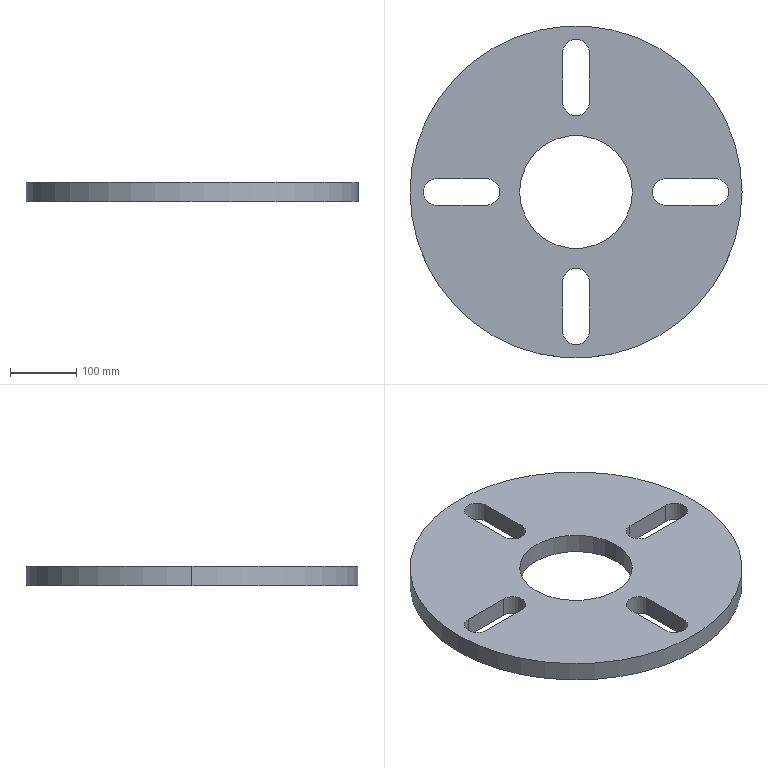Part | SolidWorks | features BaseBody 1 | 1 solid | 24 faces | box 500 x 500 x 30 mm | volume 4699230 mm3 | cylinder 14 | plane 10 | commonest cylinder face diameters 40 x10 170 x2 500 x2
STEP:
#1=CARTESIAN_POINT('',(2992.168,2025.631,30.));
#2=VERTEX_POINT('',#1);
#3=CARTESIAN_POINT('',(3162.168,2025.631,30.));
#4=VERTEX_POINT('',#3);
#5=CARTESIAN_POINT('',(3077.168,2025.631,30.));
#6=DIRECTION('',(0.,0.,1.));
#7=DIRECTION('',(1.,0.,0.));
#8=AXIS2_PLACEMENT_3D('',#5,#6,#7);
#9=CIRCLE('',#8,85.);
#10=EDGE_CURVE('',#2,#4,#9,.T.);
#11=ORIENTED_EDGE('',*,*,#10,.T.);
#12=CARTESIAN_POINT('',(3162.168,2025.631,0.));
#13=VERTEX_POINT('',#12);
#14=CARTESIAN_POINT('',(3162.168,2025.631,30.));
#15=DIRECTION('',(0.,0.,-1.));
#16=VECTOR('',#15,1000.);
#17=LINE('',#14,#16);
#18=EDGE_CURVE('',#4,#13,#17,.T.);
#19=ORIENTED_EDGE('',*,*,#18,.T.);
#20=CARTESIAN_POINT('',(2992.168,2025.631,0.));
#21=VERTEX_POINT('',#20);
#22=CARTESIAN_POINT('',(3077.168,2025.631,0.));
#23=DIRECTION('',(0.,0.,1.));
#24=DIRECTION('',(1.,0.,0.));
#25=AXIS2_PLACEMENT_3D('',#22,#23,#24);
#26=CIRCLE('',#25,85.);
#27=EDGE_CURVE('',#21,#13,#26,.T.);
#28=ORIENTED_EDGE('',*,*,#27,.F.);
#29=CARTESIAN_POINT('',(2992.168,2025.631,30.));
#30=DIRECTION('',(0.,0.,-1.));
#31=VECTOR('',#30,1000.);
#32=LINE('',#29,#31);
#33=EDGE_CURVE('',#2,#21,#32,.T.);
#34=ORIENTED_EDGE('',*,*,#33,.F.);
#35=EDGE_LOOP('',(#11,#19,#28,#34));
#36=FACE_OUTER_BOUND('',#35,.T.);
#37=CARTESIAN_POINT('',(3077.168,2025.631,30.));
#38=DIRECTION('',(0.,0.,-1.));
#39=DIRECTION('',(-1.,0.,0.));
#40=AXIS2_PLACEMENT_3D('',#37,#38,#39);
#41=CYLINDRICAL_SURFACE('',#40,85.);
#42=ADVANCED_FACE('',(#36),#41,.F.);
#43=CARTESIAN_POINT('',(3212.168,2045.62,30.));
#44=VERTEX_POINT('',#43);
#45=CARTESIAN_POINT('',(3192.168,2025.62,30.));
#46=VERTEX_POINT('',#45);
#47=CARTESIAN_POINT('',(3212.168,2025.62,30.));
#48=DIRECTION('',(0.,0.,1.));
#49=DIRECTION('',(1.,0.,0.));
#50=AXIS2_PLACEMENT_3D('',#47,#48,#49);
#51=CIRCLE('',#50,20.);
#52=EDGE_CURVE('',#44,#46,#51,.T.);
#53=ORIENTED_EDGE('',*,*,#52,.T.);
#54=CARTESIAN_POINT('',(3192.168,2025.62,0.));
#55=VERTEX_POINT('',#54);
#56=CARTESIAN_POINT('',(3192.168,2025.62,30.));
#57=DIRECTION('',(0.,0.,-1.));
#58=VECTOR('',#57,1000.);
#59=LINE('',#56,#58);
#60=EDGE_CURVE('',#46,#55,#59,.T.);
#61=ORIENTED_EDGE('',*,*,#60,.T.);
#62=CARTESIAN_POINT('',(3212.168,2045.62,0.));
#63=VERTEX_POINT('',#62);
#64=CARTESIAN_POINT('',(3212.168,2025.62,0.));
#65=DIRECTION('',(0.,0.,1.));
#66=DIRECTION('',(1.,0.,0.));
#67=AXIS2_PLACEMENT_3D('',#64,#65,#66);
#68=CIRCLE('',#67,20.);
#69=EDGE_CURVE('',#63,#55,#68,.T.);
#70=ORIENTED_EDGE('',*,*,#69,.F.);
#71=CARTESIAN_POINT('',(3212.168,2045.62,30.));
#72=DIRECTION('',(0.,0.,-1.));
#73=VECTOR('',#72,1000.);
#74=LINE('',#71,#73);
#75=EDGE_CURVE('',#44,#63,#74,.T.);
#76=ORIENTED_EDGE('',*,*,#75,.F.);
#77=EDGE_LOOP('',(#53,#61,#70,#76));
#78=FACE_OUTER_BOUND('',#77,.T.);
#79=CARTESIAN_POINT('',(3212.168,2025.62,30.));
#80=DIRECTION('',(0.,0.,-1.));
#81=DIRECTION('',(-1.,0.,0.));
#82=AXIS2_PLACEMENT_3D('',#79,#80,#81);
#83=CYLINDRICAL_SURFACE('',#82,20.);
#84=ADVANCED_FACE('',(#78),#83,.F.);
#85=CARTESIAN_POINT('',(2867.268,2045.631,30.));
#86=VERTEX_POINT('',#85);
#87=CARTESIAN_POINT('',(2847.268,2025.631,30.));
#88=VERTEX_POINT('',#87);
#89=CARTESIAN_POINT('',(2867.268,2025.631,30.));
#90=DIRECTION('',(0.,0.,1.));
#91=DIRECTION('',(1.,0.,0.));
#92=AXIS2_PLACEMENT_3D('',#89,#90,#91);
#93=CIRCLE('',#92,20.);
#94=EDGE_CURVE('',#86,#88,#93,.T.);
#95=ORIENTED_EDGE('',*,*,#94,.T.);
#96=CARTESIAN_POINT('',(2847.268,2025.631,0.));
#97=VERTEX_POINT('',#96);
#98=CARTESIAN_POINT('',(2847.268,2025.631,30.));
#99=DIRECTION('',(0.,0.,-1.));
#100=VECTOR('',#99,1000.);
#101=LINE('',#98,#100);
#102=EDGE_CURVE('',#88,#97,#101,.T.);
#103=ORIENTED_EDGE('',*,*,#102,.T.);
#104=CARTESIAN_POINT('',(2867.268,2045.631,0.));
#105=VERTEX_POINT('',#104);
#106=CARTESIAN_POINT('',(2867.268,2025.631,0.));
#107=DIRECTION('',(0.,0.,1.));
#108=DIRECTION('',(1.,0.,0.));
#109=AXIS2_PLACEMENT_3D('',#106,#107,#108);
#110=CIRCLE('',#109,20.);
#111=EDGE_CURVE('',#105,#97,#110,.T.);
#112=ORIENTED_EDGE('',*,*,#111,.F.);
#113=CARTESIAN_POINT('',(2867.268,2045.631,30.));
#114=DIRECTION('',(0.,0.,-1.));
#115=VECTOR('',#114,1000.);
#116=LINE('',#113,#115);
#117=EDGE_CURVE('',#86,#105,#116,.T.);
#118=ORIENTED_EDGE('',*,*,#117,.F.);
#119=EDGE_LOOP('',(#95,#103,#112,#118));
#120=FACE_OUTER_BOUND('',#119,.T.);
#121=CARTESIAN_POINT('',(2867.268,2025.631,30.));
#122=DIRECTION('',(0.,0.,-1.));
#123=DIRECTION('',(-1.,0.,0.));
#124=AXIS2_PLACEMENT_3D('',#121,#122,#123);
#125=CYLINDRICAL_SURFACE('',#124,20.);
#126=ADVANCED_FACE('',(#120),#125,.F.);
#127=CARTESIAN_POINT('',(3327.168,2025.631,30.));
#128=VERTEX_POINT('',#127);
#129=CARTESIAN_POINT('',(2827.168,2025.631,30.));
#130=VERTEX_POINT('',#129);
#131=CARTESIAN_POINT('',(3077.168,2025.631,30.));
#132=DIRECTION('',(0.,0.,1.));
#133=DIRECTION('',(1.,0.,0.));
#134=AXIS2_PLACEMENT_3D('',#131,#132,#133);
#135=CIRCLE('',#134,250.);
#136=EDGE_CURVE('',#128,#130,#135,.T.);
#137=ORIENTED_EDGE('',*,*,#136,.F.);
#138=CARTESIAN_POINT('',(3327.168,2025.631,0.));
#139=VERTEX_POINT('',#138);
#140=CARTESIAN_POINT('',(3327.168,2025.631,30.));
#141=DIRECTION('',(0.,0.,-1.));
#142=VECTOR('',#141,1000.);
#143=LINE('',#140,#142);
#144=EDGE_CURVE('',#128,#139,#143,.T.);
#145=ORIENTED_EDGE('',*,*,#144,.T.);
#146=CARTESIAN_POINT('',(2827.168,2025.631,0.));
#147=VERTEX_POINT('',#146);
#148=CARTESIAN_POINT('',(3077.168,2025.631,0.));
#149=DIRECTION('',(0.,0.,1.));
#150=DIRECTION('',(1.,0.,0.));
#151=AXIS2_PLACEMENT_3D('',#148,#149,#150);
#152=CIRCLE('',#151,250.);
#153=EDGE_CURVE('',#139,#147,#152,.T.);
#154=ORIENTED_EDGE('',*,*,#153,.T.);
#155=CARTESIAN_POINT('',(2827.168,2025.631,30.));
#156=DIRECTION('',(0.,0.,-1.));
#157=VECTOR('',#156,1000.);
#158=LINE('',#155,#157);
#159=EDGE_CURVE('',#130,#147,#158,.T.);
#160=ORIENTED_EDGE('',*,*,#159,.F.);
#161=EDGE_LOOP('',(#137,#145,#154,#160));
#162=FACE_OUTER_BOUND('',#161,.T.);
#163=CARTESIAN_POINT('',(3077.168,2025.631,30.));
#164=DIRECTION('',(0.,0.,-1.));
#165=DIRECTION('',(-1.,0.,0.));
#166=AXIS2_PLACEMENT_3D('',#163,#164,#165);
#167=CYLINDRICAL_SURFACE('',#166,250.);
#168=ADVANCED_FACE('',(#162),#167,.T.);
#169=CARTESIAN_POINT('',(3287.068,2045.631,30.));
#170=VERTEX_POINT('',#169);
#171=CARTESIAN_POINT('',(3287.068,2045.631,30.));
#172=DIRECTION('',(-1.,-0.0001515,0.));
#173=VECTOR('',#172,1000.);
#174=LINE('',#171,#173);
#175=EDGE_CURVE('',#170,#44,#174,.T.);
#176=ORIENTED_EDGE('',*,*,#175,.F.);
#177=CARTESIAN_POINT('',(3287.068,2005.631,30.));
#178=VERTEX_POINT('',#177);
#179=CARTESIAN_POINT('',(3287.068,2025.631,30.));
#180=DIRECTION('',(0.,0.,1.));
#181=DIRECTION('',(1.,0.,0.));
#182=AXIS2_PLACEMENT_3D('',#179,#180,#181);
#183=CIRCLE('',#182,20.);
#184=EDGE_CURVE('',#178,#170,#183,.T.);
#185=ORIENTED_EDGE('',*,*,#184,.F.);
#186=CARTESIAN_POINT('',(3212.168,2005.62,30.));
#187=VERTEX_POINT('',#186);
#188=CARTESIAN_POINT('',(3287.068,2005.631,30.));
#189=DIRECTION('',(1.,0.0001515,0.));
#190=VECTOR('',#189,1000.);
#191=LINE('',#188,#190);
#192=EDGE_CURVE('',#187,#178,#191,.T.);
#193=ORIENTED_EDGE('',*,*,#192,.F.);
#194=CARTESIAN_POINT('',(3212.168,2025.62,30.));
#195=DIRECTION('',(0.,0.,1.));
#196=DIRECTION('',(1.,0.,0.));
#197=AXIS2_PLACEMENT_3D('',#194,#195,#196);
#198=CIRCLE('',#197,20.);
#199=EDGE_CURVE('',#46,#187,#198,.T.);
#200=ORIENTED_EDGE('',*,*,#199,.F.);
#201=ORIENTED_EDGE('',*,*,#52,.F.);
#202=EDGE_LOOP('',(#176,#185,#193,#200,#201));
#203=FACE_BOUND('',#202,.T.);
#204=CARTESIAN_POINT('',(3097.168,1815.731,30.));
#205=VERTEX_POINT('',#204);
#206=CARTESIAN_POINT('',(3097.157,1890.631,30.));
#207=VERTEX_POINT('',#206);
#208=CARTESIAN_POINT('',(3097.168,1815.731,30.));
#209=DIRECTION('',(-0.0001515,1.,0.));
#210=VECTOR('',#209,1000.);
#211=LINE('',#208,#210);
#212=EDGE_CURVE('',#205,#207,#211,.T.);
#213=ORIENTED_EDGE('',*,*,#212,.F.);
#214=CARTESIAN_POINT('',(3057.168,1815.731,30.));
#215=VERTEX_POINT('',#214);
#216=CARTESIAN_POINT('',(3077.168,1815.731,30.));
#217=DIRECTION('',(0.,0.,1.));
#218=DIRECTION('',(1.,0.,0.));
#219=AXIS2_PLACEMENT_3D('',#216,#217,#218);
#220=CIRCLE('',#219,20.);
#221=EDGE_CURVE('',#215,#205,#220,.T.);
#222=ORIENTED_EDGE('',*,*,#221,.F.);
#223=CARTESIAN_POINT('',(3057.157,1890.631,30.));
#224=VERTEX_POINT('',#223);
#225=CARTESIAN_POINT('',(3057.168,1815.731,30.));
#226=DIRECTION('',(0.0001515,-1.,0.));
#227=VECTOR('',#226,1000.);
#228=LINE('',#225,#227);
#229=EDGE_CURVE('',#224,#215,#228,.T.);
#230=ORIENTED_EDGE('',*,*,#229,.F.);
#231=CARTESIAN_POINT('',(3077.157,1890.631,30.));
#232=DIRECTION('',(0.,0.,1.));
#233=DIRECTION('',(1.,0.,0.));
#234=AXIS2_PLACEMENT_3D('',#231,#232,#233);
#235=CIRCLE('',#234,20.);
#236=EDGE_CURVE('',#207,#224,#235,.T.);
#237=ORIENTED_EDGE('',*,*,#236,.F.);
#238=EDGE_LOOP('',(#213,#222,#230,#237));
#239=FACE_BOUND('',#238,.T.);
#240=CARTESIAN_POINT('',(2867.268,2005.631,30.));
#241=VERTEX_POINT('',#240);
#242=CARTESIAN_POINT('',(2942.168,2005.643,30.));
#243=VERTEX_POINT('',#242);
#244=CARTESIAN_POINT('',(2867.268,2005.631,30.));
#245=DIRECTION('',(1.,0.0001515,0.));
#246=VECTOR('',#245,1000.);
#247=LINE('',#244,#246);
#248=EDGE_CURVE('',#241,#243,#247,.T.);
#249=ORIENTED_EDGE('',*,*,#248,.F.);
#250=CARTESIAN_POINT('',(2867.268,2025.631,30.));
#251=DIRECTION('',(0.,0.,1.));
#252=DIRECTION('',(1.,0.,0.));
#253=AXIS2_PLACEMENT_3D('',#250,#251,#252);
#254=CIRCLE('',#253,20.);
#255=EDGE_CURVE('',#88,#241,#254,.T.);
#256=ORIENTED_EDGE('',*,*,#255,.F.);
#257=ORIENTED_EDGE('',*,*,#94,.F.);
#258=CARTESIAN_POINT('',(2942.168,2045.643,30.));
#259=VERTEX_POINT('',#258);
#260=CARTESIAN_POINT('',(2867.268,2045.631,30.));
#261=DIRECTION('',(-1.,-0.0001515,0.));
#262=VECTOR('',#261,1000.);
#263=LINE('',#260,#262);
#264=EDGE_CURVE('',#259,#86,#263,.T.);
#265=ORIENTED_EDGE('',*,*,#264,.F.);
#266=CARTESIAN_POINT('',(2942.168,2025.643,30.));
#267=DIRECTION('',(0.,0.,1.));
#268=DIRECTION('',(1.,0.,0.));
#269=AXIS2_PLACEMENT_3D('',#266,#267,#268);
#270=CIRCLE('',#269,20.);
#271=EDGE_CURVE('',#243,#259,#270,.T.);
#272=ORIENTED_EDGE('',*,*,#271,.F.);
#273=EDGE_LOOP('',(#249,#256,#257,#265,#272));
#274=FACE_BOUND('',#273,.T.);
#275=CARTESIAN_POINT('',(3057.168,2235.531,30.));
#276=VERTEX_POINT('',#275);
#277=CARTESIAN_POINT('',(3057.18,2160.631,30.));
#278=VERTEX_POINT('',#277);
#279=CARTESIAN_POINT('',(3057.168,2235.531,30.));
#280=DIRECTION('',(0.0001515,-1.,0.));
#281=VECTOR('',#280,1000.);
#282=LINE('',#279,#281);
#283=EDGE_CURVE('',#276,#278,#282,.T.);
#284=ORIENTED_EDGE('',*,*,#283,.F.);
#285=CARTESIAN_POINT('',(3097.168,2235.531,30.));
#286=VERTEX_POINT('',#285);
#287=CARTESIAN_POINT('',(3077.168,2235.531,30.));
#288=DIRECTION('',(0.,0.,1.));
#289=DIRECTION('',(1.,0.,0.));
#290=AXIS2_PLACEMENT_3D('',#287,#288,#289);
#291=CIRCLE('',#290,20.);
#292=EDGE_CURVE('',#286,#276,#291,.T.);
#293=ORIENTED_EDGE('',*,*,#292,.F.);
#294=CARTESIAN_POINT('',(3097.18,2160.631,30.));
#295=VERTEX_POINT('',#294);
#296=CARTESIAN_POINT('',(3097.168,2235.531,30.));
#297=DIRECTION('',(-0.0001515,1.,0.));
#298=VECTOR('',#297,1000.);
#299=LINE('',#296,#298);
#300=EDGE_CURVE('',#295,#286,#299,.T.);
#301=ORIENTED_EDGE('',*,*,#300,.F.);
#302=CARTESIAN_POINT('',(3077.18,2160.631,30.));
#303=DIRECTION('',(0.,0.,1.));
#304=DIRECTION('',(1.,0.,0.));
#305=AXIS2_PLACEMENT_3D('',#302,#303,#304);
#306=CIRCLE('',#305,20.);
#307=EDGE_CURVE('',#278,#295,#306,.T.);
#308=ORIENTED_EDGE('',*,*,#307,.F.);
#309=EDGE_LOOP('',(#284,#293,#301,#308));
#310=FACE_BOUND('',#309,.T.);
#311=CARTESIAN_POINT('',(3077.168,2025.631,30.));
#312=DIRECTION('',(0.,0.,1.));
#313=DIRECTION('',(1.,0.,0.));
#314=AXIS2_PLACEMENT_3D('',#311,#312,#313);
#315=CIRCLE('',#314,250.);
#316=EDGE_CURVE('',#130,#128,#315,.T.);
#317=ORIENTED_EDGE('',*,*,#316,.T.);
#318=ORIENTED_EDGE('',*,*,#136,.T.);
#319=EDGE_LOOP('',(#317,#318));
#320=FACE_OUTER_BOUND('',#319,.T.);
#321=ORIENTED_EDGE('',*,*,#10,.F.);
#322=CARTESIAN_POINT('',(3077.168,2025.631,30.));
#323=DIRECTION('',(0.,0.,1.));
#324=DIRECTION('',(1.,0.,0.));
#325=AXIS2_PLACEMENT_3D('',#322,#323,#324);
#326=CIRCLE('',#325,85.);
#327=EDGE_CURVE('',#4,#2,#326,.T.);
#328=ORIENTED_EDGE('',*,*,#327,.F.);
#329=EDGE_LOOP('',(#321,#328));
#330=FACE_BOUND('',#329,.T.);
#331=CARTESIAN_POINT('',(3077.168,2025.631,30.));
#332=DIRECTION('',(0.,0.,1.));
#333=DIRECTION('',(1.,0.,0.));
#334=AXIS2_PLACEMENT_3D('',#331,#332,#333);
#335=PLANE('',#334);
#336=ADVANCED_FACE('',(#203,#239,#274,#310,#320,#330),#335,.T.);
#337=CARTESIAN_POINT('',(3057.168,1815.731,0.));
#338=VERTEX_POINT('',#337);
#339=CARTESIAN_POINT('',(3097.168,1815.731,0.));
#340=VERTEX_POINT('',#339);
#341=CARTESIAN_POINT('',(3077.168,1815.731,0.));
#342=DIRECTION('',(0.,0.,1.));
#343=DIRECTION('',(1.,0.,0.));
#344=AXIS2_PLACEMENT_3D('',#341,#342,#343);
#345=CIRCLE('',#344,20.);
#346=EDGE_CURVE('',#338,#340,#345,.T.);
#347=ORIENTED_EDGE('',*,*,#346,.T.);
#348=CARTESIAN_POINT('',(3097.157,1890.631,0.));
#349=VERTEX_POINT('',#348);
#350=CARTESIAN_POINT('',(3097.168,1815.731,0.));
#351=DIRECTION('',(-0.0001515,1.,0.));
#352=VECTOR('',#351,1000.);
#353=LINE('',#350,#352);
#354=EDGE_CURVE('',#340,#349,#353,.T.);
#355=ORIENTED_EDGE('',*,*,#354,.T.);
#356=CARTESIAN_POINT('',(3057.157,1890.631,0.));
#357=VERTEX_POINT('',#356);
#358=CARTESIAN_POINT('',(3077.157,1890.631,0.));
#359=DIRECTION('',(0.,0.,1.));
#360=DIRECTION('',(1.,0.,0.));
#361=AXIS2_PLACEMENT_3D('',#358,#359,#360);
#362=CIRCLE('',#361,20.);
#363=EDGE_CURVE('',#349,#357,#362,.T.);
#364=ORIENTED_EDGE('',*,*,#363,.T.);
#365=CARTESIAN_POINT('',(3057.168,1815.731,0.));
#366=DIRECTION('',(0.0001515,-1.,0.));
#367=VECTOR('',#366,1000.);
#368=LINE('',#365,#367);
#369=EDGE_CURVE('',#357,#338,#368,.T.);
#370=ORIENTED_EDGE('',*,*,#369,.T.);
#371=EDGE_LOOP('',(#347,#355,#364,#370));
#372=FACE_BOUND('',#371,.T.);
#373=CARTESIAN_POINT('',(3097.168,2235.531,0.));
#374=VERTEX_POINT('',#373);
#375=CARTESIAN_POINT('',(3057.168,2235.531,0.));
#376=VERTEX_POINT('',#375);
#377=CARTESIAN_POINT('',(3077.168,2235.531,0.));
#378=DIRECTION('',(0.,0.,1.));
#379=DIRECTION('',(1.,0.,0.));
#380=AXIS2_PLACEMENT_3D('',#377,#378,#379);
#381=CIRCLE('',#380,20.);
#382=EDGE_CURVE('',#374,#376,#381,.T.);
#383=ORIENTED_EDGE('',*,*,#382,.T.);
#384=CARTESIAN_POINT('',(3057.18,2160.631,0.));
#385=VERTEX_POINT('',#384);
#386=CARTESIAN_POINT('',(3057.168,2235.531,0.));
#387=DIRECTION('',(0.0001515,-1.,0.));
#388=VECTOR('',#387,1000.);
#389=LINE('',#386,#388);
#390=EDGE_CURVE('',#376,#385,#389,.T.);
#391=ORIENTED_EDGE('',*,*,#390,.T.);
#392=CARTESIAN_POINT('',(3097.18,2160.631,0.));
#393=VERTEX_POINT('',#392);
#394=CARTESIAN_POINT('',(3077.18,2160.631,0.));
#395=DIRECTION('',(0.,0.,1.));
#396=DIRECTION('',(1.,0.,0.));
#397=AXIS2_PLACEMENT_3D('',#394,#395,#396);
#398=CIRCLE('',#397,20.);
#399=EDGE_CURVE('',#385,#393,#398,.T.);
#400=ORIENTED_EDGE('',*,*,#399,.T.);
#401=CARTESIAN_POINT('',(3097.168,2235.531,0.));
#402=DIRECTION('',(-0.0001515,1.,0.));
#403=VECTOR('',#402,1000.);
#404=LINE('',#401,#403);
#405=EDGE_CURVE('',#393,#374,#404,.T.);
#406=ORIENTED_EDGE('',*,*,#405,.T.);
#407=EDGE_LOOP('',(#383,#391,#400,#406));
#408=FACE_BOUND('',#407,.T.);
#409=CARTESIAN_POINT('',(3077.168,2025.631,0.));
#410=DIRECTION('',(0.,0.,1.));
#411=DIRECTION('',(1.,0.,0.));
#412=AXIS2_PLACEMENT_3D('',#409,#410,#411);
#413=CIRCLE('',#412,250.);
#414=EDGE_CURVE('',#147,#139,#413,.T.);
#415=ORIENTED_EDGE('',*,*,#414,.F.);
#416=ORIENTED_EDGE('',*,*,#153,.F.);
#417=EDGE_LOOP('',(#415,#416));
#418=FACE_OUTER_BOUND('',#417,.T.);
#419=ORIENTED_EDGE('',*,*,#111,.T.);
#420=CARTESIAN_POINT('',(2867.268,2005.631,0.));
#421=VERTEX_POINT('',#420);
#422=CARTESIAN_POINT('',(2867.268,2025.631,0.));
#423=DIRECTION('',(0.,0.,1.));
#424=DIRECTION('',(1.,0.,0.));
#425=AXIS2_PLACEMENT_3D('',#422,#423,#424);
#426=CIRCLE('',#425,20.);
#427=EDGE_CURVE('',#97,#421,#426,.T.);
#428=ORIENTED_EDGE('',*,*,#427,.T.);
#429=CARTESIAN_POINT('',(2942.168,2005.643,0.));
#430=VERTEX_POINT('',#429);
#431=CARTESIAN_POINT('',(2867.268,2005.631,0.));
#432=DIRECTION('',(1.,0.0001515,0.));
#433=VECTOR('',#432,1000.);
#434=LINE('',#431,#433);
#435=EDGE_CURVE('',#421,#430,#434,.T.);
#436=ORIENTED_EDGE('',*,*,#435,.T.);
#437=CARTESIAN_POINT('',(2942.168,2045.643,0.));
#438=VERTEX_POINT('',#437);
#439=CARTESIAN_POINT('',(2942.168,2025.643,0.));
#440=DIRECTION('',(0.,0.,1.));
#441=DIRECTION('',(1.,0.,0.));
#442=AXIS2_PLACEMENT_3D('',#439,#440,#441);
#443=CIRCLE('',#442,20.);
#444=EDGE_CURVE('',#430,#438,#443,.T.);
#445=ORIENTED_EDGE('',*,*,#444,.T.);
#446=CARTESIAN_POINT('',(2867.268,2045.631,0.));
#447=DIRECTION('',(-1.,-0.0001515,0.));
#448=VECTOR('',#447,1000.);
#449=LINE('',#446,#448);
#450=EDGE_CURVE('',#438,#105,#449,.T.);
#451=ORIENTED_EDGE('',*,*,#450,.T.);
#452=EDGE_LOOP('',(#419,#428,#436,#445,#451));
#453=FACE_BOUND('',#452,.T.);
#454=CARTESIAN_POINT('',(3287.068,2005.631,0.));
#455=VERTEX_POINT('',#454);
#456=CARTESIAN_POINT('',(3287.068,2045.631,0.));
#457=VERTEX_POINT('',#456);
#458=CARTESIAN_POINT('',(3287.068,2025.631,0.));
#459=DIRECTION('',(0.,0.,1.));
#460=DIRECTION('',(1.,0.,0.));
#461=AXIS2_PLACEMENT_3D('',#458,#459,#460);
#462=CIRCLE('',#461,20.);
#463=EDGE_CURVE('',#455,#457,#462,.T.);
#464=ORIENTED_EDGE('',*,*,#463,.T.);
#465=CARTESIAN_POINT('',(3287.068,2045.631,0.));
#466=DIRECTION('',(-1.,-0.0001515,0.));
#467=VECTOR('',#466,1000.);
#468=LINE('',#465,#467);
#469=EDGE_CURVE('',#457,#63,#468,.T.);
#470=ORIENTED_EDGE('',*,*,#469,.T.);
#471=ORIENTED_EDGE('',*,*,#69,.T.);
#472=CARTESIAN_POINT('',(3212.168,2005.62,0.));
#473=VERTEX_POINT('',#472);
#474=CARTESIAN_POINT('',(3212.168,2025.62,0.));
#475=DIRECTION('',(0.,0.,1.));
#476=DIRECTION('',(1.,0.,0.));
#477=AXIS2_PLACEMENT_3D('',#474,#475,#476);
#478=CIRCLE('',#477,20.);
#479=EDGE_CURVE('',#55,#473,#478,.T.);
#480=ORIENTED_EDGE('',*,*,#479,.T.);
#481=CARTESIAN_POINT('',(3287.068,2005.631,0.));
#482=DIRECTION('',(1.,0.0001515,0.));
#483=VECTOR('',#482,1000.);
#484=LINE('',#481,#483);
#485=EDGE_CURVE('',#473,#455,#484,.T.);
#486=ORIENTED_EDGE('',*,*,#485,.T.);
#487=EDGE_LOOP('',(#464,#470,#471,#480,#486));
#488=FACE_BOUND('',#487,.T.);
#489=ORIENTED_EDGE('',*,*,#27,.T.);
#490=CARTESIAN_POINT('',(3077.168,2025.631,0.));
#491=DIRECTION('',(0.,0.,1.));
#492=DIRECTION('',(1.,0.,0.));
#493=AXIS2_PLACEMENT_3D('',#490,#491,#492);
#494=CIRCLE('',#493,85.);
#495=EDGE_CURVE('',#13,#21,#494,.T.);
#496=ORIENTED_EDGE('',*,*,#495,.T.);
#497=EDGE_LOOP('',(#489,#496));
#498=FACE_BOUND('',#497,.T.);
#499=CARTESIAN_POINT('',(3077.168,2025.631,0.));
#500=DIRECTION('',(0.,0.,1.));
#501=DIRECTION('',(1.,0.,0.));
#502=AXIS2_PLACEMENT_3D('',#499,#500,#501);
#503=PLANE('',#502);
#504=ADVANCED_FACE('',(#372,#408,#418,#453,#488,#498),#503,.F.);
#505=ORIENTED_EDGE('',*,*,#144,.F.);
#506=ORIENTED_EDGE('',*,*,#316,.F.);
#507=ORIENTED_EDGE('',*,*,#159,.T.);
#508=ORIENTED_EDGE('',*,*,#414,.T.);
#509=EDGE_LOOP('',(#505,#506,#507,#508));
#510=FACE_OUTER_BOUND('',#509,.T.);
#511=CARTESIAN_POINT('',(3077.168,2025.631,30.));
#512=DIRECTION('',(0.,0.,-1.));
#513=DIRECTION('',(-1.,0.,0.));
#514=AXIS2_PLACEMENT_3D('',#511,#512,#513);
#515=CYLINDRICAL_SURFACE('',#514,250.);
#516=ADVANCED_FACE('',(#510),#515,.T.);
#517=ORIENTED_EDGE('',*,*,#382,.F.);
#518=CARTESIAN_POINT('',(3097.168,2235.531,30.));
#519=DIRECTION('',(0.,0.,-1.));
#520=VECTOR('',#519,1000.);
#521=LINE('',#518,#520);
#522=EDGE_CURVE('',#286,#374,#521,.T.);
#523=ORIENTED_EDGE('',*,*,#522,.F.);
#524=ORIENTED_EDGE('',*,*,#292,.T.);
#525=CARTESIAN_POINT('',(3057.168,2235.531,30.));
#526=DIRECTION('',(0.,0.,-1.));
#527=VECTOR('',#526,1000.);
#528=LINE('',#525,#527);
#529=EDGE_CURVE('',#276,#376,#528,.T.);
#530=ORIENTED_EDGE('',*,*,#529,.T.);
#531=EDGE_LOOP('',(#517,#523,#524,#530));
#532=FACE_OUTER_BOUND('',#531,.T.);
#533=CARTESIAN_POINT('',(3077.168,2235.531,30.));
#534=DIRECTION('',(0.,0.,-1.));
#535=DIRECTION('',(-1.,0.,0.));
#536=AXIS2_PLACEMENT_3D('',#533,#534,#535);
#537=CYLINDRICAL_SURFACE('',#536,20.);
#538=ADVANCED_FACE('',(#532),#537,.F.);
#539=ORIENTED_EDGE('',*,*,#390,.F.);
#540=ORIENTED_EDGE('',*,*,#529,.F.);
#541=ORIENTED_EDGE('',*,*,#283,.T.);
#542=CARTESIAN_POINT('',(3057.18,2160.631,30.));
#543=DIRECTION('',(0.,0.,-1.));
#544=VECTOR('',#543,1000.);
#545=LINE('',#542,#544);
#546=EDGE_CURVE('',#278,#385,#545,.T.);
#547=ORIENTED_EDGE('',*,*,#546,.T.);
#548=EDGE_LOOP('',(#539,#540,#541,#547));
#549=FACE_OUTER_BOUND('',#548,.T.);
#550=CARTESIAN_POINT('',(3057.168,2235.531,30.));
#551=DIRECTION('',(1.,0.0001515,0.));
#552=DIRECTION('',(-0.0001515,1.,0.));
#553=AXIS2_PLACEMENT_3D('',#550,#551,#552);
#554=PLANE('',#553);
#555=ADVANCED_FACE('',(#549),#554,.T.);
#556=ORIENTED_EDGE('',*,*,#399,.F.);
#557=ORIENTED_EDGE('',*,*,#546,.F.);
#558=ORIENTED_EDGE('',*,*,#307,.T.);
#559=CARTESIAN_POINT('',(3097.18,2160.631,30.));
#560=DIRECTION('',(0.,0.,-1.));
#561=VECTOR('',#560,1000.);
#562=LINE('',#559,#561);
#563=EDGE_CURVE('',#295,#393,#562,.T.);
#564=ORIENTED_EDGE('',*,*,#563,.T.);
#565=EDGE_LOOP('',(#556,#557,#558,#564));
#566=FACE_OUTER_BOUND('',#565,.T.);
#567=CARTESIAN_POINT('',(3077.18,2160.631,30.));
#568=DIRECTION('',(0.,0.,-1.));
#569=DIRECTION('',(-1.,0.,0.));
#570=AXIS2_PLACEMENT_3D('',#567,#568,#569);
#571=CYLINDRICAL_SURFACE('',#570,20.);
#572=ADVANCED_FACE('',(#566),#571,.F.);
#573=ORIENTED_EDGE('',*,*,#405,.F.);
#574=ORIENTED_EDGE('',*,*,#563,.F.);
#575=ORIENTED_EDGE('',*,*,#300,.T.);
#576=ORIENTED_EDGE('',*,*,#522,.T.);
#577=EDGE_LOOP('',(#573,#574,#575,#576));
#578=FACE_OUTER_BOUND('',#577,.T.);
#579=CARTESIAN_POINT('',(3097.168,2235.531,30.));
#580=DIRECTION('',(-1.,-0.0001515,0.));
#581=DIRECTION('',(0.0001515,-1.,0.));
#582=AXIS2_PLACEMENT_3D('',#579,#580,#581);
#583=PLANE('',#582);
#584=ADVANCED_FACE('',(#578),#583,.T.);
#585=ORIENTED_EDGE('',*,*,#102,.F.);
#586=ORIENTED_EDGE('',*,*,#255,.T.);
#587=CARTESIAN_POINT('',(2867.268,2005.631,30.));
#588=DIRECTION('',(0.,0.,-1.));
#589=VECTOR('',#588,1000.);
#590=LINE('',#587,#589);
#591=EDGE_CURVE('',#241,#421,#590,.T.);
#592=ORIENTED_EDGE('',*,*,#591,.T.);
#593=ORIENTED_EDGE('',*,*,#427,.F.);
#594=EDGE_LOOP('',(#585,#586,#592,#593));
#595=FACE_OUTER_BOUND('',#594,.T.);
#596=CARTESIAN_POINT('',(2867.268,2025.631,30.));
#597=DIRECTION('',(0.,0.,-1.));
#598=DIRECTION('',(-1.,0.,0.));
#599=AXIS2_PLACEMENT_3D('',#596,#597,#598);
#600=CYLINDRICAL_SURFACE('',#599,20.);
#601=ADVANCED_FACE('',(#595),#600,.F.);
#602=ORIENTED_EDGE('',*,*,#435,.F.);
#603=ORIENTED_EDGE('',*,*,#591,.F.);
#604=ORIENTED_EDGE('',*,*,#248,.T.);
#605=CARTESIAN_POINT('',(2942.168,2005.643,30.));
#606=DIRECTION('',(0.,0.,-1.));
#607=VECTOR('',#606,1000.);
#608=LINE('',#605,#607);
#609=EDGE_CURVE('',#243,#430,#608,.T.);
#610=ORIENTED_EDGE('',*,*,#609,.T.);
#611=EDGE_LOOP('',(#602,#603,#604,#610));
#612=FACE_OUTER_BOUND('',#611,.T.);
#613=CARTESIAN_POINT('',(2867.268,2005.631,30.));
#614=DIRECTION('',(-0.0001515,1.,0.));
#615=DIRECTION('',(-1.,-0.0001515,0.));
#616=AXIS2_PLACEMENT_3D('',#613,#614,#615);
#617=PLANE('',#616);
#618=ADVANCED_FACE('',(#612),#617,.T.);
#619=ORIENTED_EDGE('',*,*,#444,.F.);
#620=ORIENTED_EDGE('',*,*,#609,.F.);
#621=ORIENTED_EDGE('',*,*,#271,.T.);
#622=CARTESIAN_POINT('',(2942.168,2045.643,30.));
#623=DIRECTION('',(0.,0.,-1.));
#624=VECTOR('',#623,1000.);
#625=LINE('',#622,#624);
#626=EDGE_CURVE('',#259,#438,#625,.T.);
#627=ORIENTED_EDGE('',*,*,#626,.T.);
#628=EDGE_LOOP('',(#619,#620,#621,#627));
#629=FACE_OUTER_BOUND('',#628,.T.);
#630=CARTESIAN_POINT('',(2942.168,2025.643,30.));
#631=DIRECTION('',(0.,0.,-1.));
#632=DIRECTION('',(-1.,0.,0.));
#633=AXIS2_PLACEMENT_3D('',#630,#631,#632);
#634=CYLINDRICAL_SURFACE('',#633,20.);
#635=ADVANCED_FACE('',(#629),#634,.F.);
#636=ORIENTED_EDGE('',*,*,#450,.F.);
#637=ORIENTED_EDGE('',*,*,#626,.F.);
#638=ORIENTED_EDGE('',*,*,#264,.T.);
#639=ORIENTED_EDGE('',*,*,#117,.T.);
#640=EDGE_LOOP('',(#636,#637,#638,#639));
#641=FACE_OUTER_BOUND('',#640,.T.);
#642=CARTESIAN_POINT('',(2867.268,2045.631,30.));
#643=DIRECTION('',(0.0001515,-1.,0.));
#644=DIRECTION('',(1.,0.0001515,0.));
#645=AXIS2_PLACEMENT_3D('',#642,#643,#644);
#646=PLANE('',#645);
#647=ADVANCED_FACE('',(#641),#646,.T.);
#648=ORIENTED_EDGE('',*,*,#346,.F.);
#649=CARTESIAN_POINT('',(3057.168,1815.731,30.));
#650=DIRECTION('',(0.,0.,-1.));
#651=VECTOR('',#650,1000.);
#652=LINE('',#649,#651);
#653=EDGE_CURVE('',#215,#338,#652,.T.);
#654=ORIENTED_EDGE('',*,*,#653,.F.);
#655=ORIENTED_EDGE('',*,*,#221,.T.);
#656=CARTESIAN_POINT('',(3097.168,1815.731,30.));
#657=DIRECTION('',(0.,0.,-1.));
#658=VECTOR('',#657,1000.);
#659=LINE('',#656,#658);
#660=EDGE_CURVE('',#205,#340,#659,.T.);
#661=ORIENTED_EDGE('',*,*,#660,.T.);
#662=EDGE_LOOP('',(#648,#654,#655,#661));
#663=FACE_OUTER_BOUND('',#662,.T.);
#664=CARTESIAN_POINT('',(3077.168,1815.731,30.));
#665=DIRECTION('',(0.,0.,-1.));
#666=DIRECTION('',(-1.,0.,0.));
#667=AXIS2_PLACEMENT_3D('',#664,#665,#666);
#668=CYLINDRICAL_SURFACE('',#667,20.);
#669=ADVANCED_FACE('',(#663),#668,.F.);
#670=ORIENTED_EDGE('',*,*,#354,.F.);
#671=ORIENTED_EDGE('',*,*,#660,.F.);
#672=ORIENTED_EDGE('',*,*,#212,.T.);
#673=CARTESIAN_POINT('',(3097.157,1890.631,30.));
#674=DIRECTION('',(0.,0.,-1.));
#675=VECTOR('',#674,1000.);
#676=LINE('',#673,#675);
#677=EDGE_CURVE('',#207,#349,#676,.T.);
#678=ORIENTED_EDGE('',*,*,#677,.T.);
#679=EDGE_LOOP('',(#670,#671,#672,#678));
#680=FACE_OUTER_BOUND('',#679,.T.);
#681=CARTESIAN_POINT('',(3097.168,1815.731,30.));
#682=DIRECTION('',(-1.,-0.0001515,0.));
#683=DIRECTION('',(0.0001515,-1.,0.));
#684=AXIS2_PLACEMENT_3D('',#681,#682,#683);
#685=PLANE('',#684);
#686=ADVANCED_FACE('',(#680),#685,.T.);
#687=ORIENTED_EDGE('',*,*,#363,.F.);
#688=ORIENTED_EDGE('',*,*,#677,.F.);
#689=ORIENTED_EDGE('',*,*,#236,.T.);
#690=CARTESIAN_POINT('',(3057.157,1890.631,30.));
#691=DIRECTION('',(0.,0.,-1.));
#692=VECTOR('',#691,1000.);
#693=LINE('',#690,#692);
#694=EDGE_CURVE('',#224,#357,#693,.T.);
#695=ORIENTED_EDGE('',*,*,#694,.T.);
#696=EDGE_LOOP('',(#687,#688,#689,#695));
#697=FACE_OUTER_BOUND('',#696,.T.);
#698=CARTESIAN_POINT('',(3077.157,1890.631,30.));
#699=DIRECTION('',(0.,0.,-1.));
#700=DIRECTION('',(-1.,0.,0.));
#701=AXIS2_PLACEMENT_3D('',#698,#699,#700);
#702=CYLINDRICAL_SURFACE('',#701,20.);
#703=ADVANCED_FACE('',(#697),#702,.F.);
#704=ORIENTED_EDGE('',*,*,#369,.F.);
#705=ORIENTED_EDGE('',*,*,#694,.F.);
#706=ORIENTED_EDGE('',*,*,#229,.T.);
#707=ORIENTED_EDGE('',*,*,#653,.T.);
#708=EDGE_LOOP('',(#704,#705,#706,#707));
#709=FACE_OUTER_BOUND('',#708,.T.);
#710=CARTESIAN_POINT('',(3057.168,1815.731,30.));
#711=DIRECTION('',(1.,0.0001515,0.));
#712=DIRECTION('',(-0.0001515,1.,0.));
#713=AXIS2_PLACEMENT_3D('',#710,#711,#712);
#714=PLANE('',#713);
#715=ADVANCED_FACE('',(#709),#714,.T.);
#716=ORIENTED_EDGE('',*,*,#463,.F.);
#717=CARTESIAN_POINT('',(3287.068,2005.631,30.));
#718=DIRECTION('',(0.,0.,-1.));
#719=VECTOR('',#718,1000.);
#720=LINE('',#717,#719);
#721=EDGE_CURVE('',#178,#455,#720,.T.);
#722=ORIENTED_EDGE('',*,*,#721,.F.);
#723=ORIENTED_EDGE('',*,*,#184,.T.);
#724=CARTESIAN_POINT('',(3287.068,2045.631,30.));
#725=DIRECTION('',(0.,0.,-1.));
#726=VECTOR('',#725,1000.);
#727=LINE('',#724,#726);
#728=EDGE_CURVE('',#170,#457,#727,.T.);
#729=ORIENTED_EDGE('',*,*,#728,.T.);
#730=EDGE_LOOP('',(#716,#722,#723,#729));
#731=FACE_OUTER_BOUND('',#730,.T.);
#732=CARTESIAN_POINT('',(3287.068,2025.631,30.));
#733=DIRECTION('',(0.,0.,-1.));
#734=DIRECTION('',(-1.,0.,0.));
#735=AXIS2_PLACEMENT_3D('',#732,#733,#734);
#736=CYLINDRICAL_SURFACE('',#735,20.);
#737=ADVANCED_FACE('',(#731),#736,.F.);
#738=ORIENTED_EDGE('',*,*,#469,.F.);
#739=ORIENTED_EDGE('',*,*,#728,.F.);
#740=ORIENTED_EDGE('',*,*,#175,.T.);
#741=ORIENTED_EDGE('',*,*,#75,.T.);
#742=EDGE_LOOP('',(#738,#739,#740,#741));
#743=FACE_OUTER_BOUND('',#742,.T.);
#744=CARTESIAN_POINT('',(3287.068,2045.631,30.));
#745=DIRECTION('',(0.0001515,-1.,0.));
#746=DIRECTION('',(1.,0.0001515,0.));
#747=AXIS2_PLACEMENT_3D('',#744,#745,#746);
#748=PLANE('',#747);
#749=ADVANCED_FACE('',(#743),#748,.T.);
#750=ORIENTED_EDGE('',*,*,#60,.F.);
#751=ORIENTED_EDGE('',*,*,#199,.T.);
#752=CARTESIAN_POINT('',(3212.168,2005.62,30.));
#753=DIRECTION('',(0.,0.,-1.));
#754=VECTOR('',#753,1000.);
#755=LINE('',#752,#754);
#756=EDGE_CURVE('',#187,#473,#755,.T.);
#757=ORIENTED_EDGE('',*,*,#756,.T.);
#758=ORIENTED_EDGE('',*,*,#479,.F.);
#759=EDGE_LOOP('',(#750,#751,#757,#758));
#760=FACE_OUTER_BOUND('',#759,.T.);
#761=CARTESIAN_POINT('',(3212.168,2025.62,30.));
#762=DIRECTION('',(0.,0.,-1.));
#763=DIRECTION('',(-1.,0.,0.));
#764=AXIS2_PLACEMENT_3D('',#761,#762,#763);
#765=CYLINDRICAL_SURFACE('',#764,20.);
#766=ADVANCED_FACE('',(#760),#765,.F.);
#767=ORIENTED_EDGE('',*,*,#485,.F.);
#768=ORIENTED_EDGE('',*,*,#756,.F.);
#769=ORIENTED_EDGE('',*,*,#192,.T.);
#770=ORIENTED_EDGE('',*,*,#721,.T.);
#771=EDGE_LOOP('',(#767,#768,#769,#770));
#772=FACE_OUTER_BOUND('',#771,.T.);
#773=CARTESIAN_POINT('',(3287.068,2005.631,30.));
#774=DIRECTION('',(-0.0001515,1.,0.));
#775=DIRECTION('',(-1.,-0.0001515,0.));
#776=AXIS2_PLACEMENT_3D('',#773,#774,#775);
#777=PLANE('',#776);
#778=ADVANCED_FACE('',(#772),#777,.T.);
#779=ORIENTED_EDGE('',*,*,#18,.F.);
#780=ORIENTED_EDGE('',*,*,#327,.T.);
#781=ORIENTED_EDGE('',*,*,#33,.T.);
#782=ORIENTED_EDGE('',*,*,#495,.F.);
#783=EDGE_LOOP('',(#779,#780,#781,#782));
#784=FACE_OUTER_BOUND('',#783,.T.);
#785=CARTESIAN_POINT('',(3077.168,2025.631,30.));
#786=DIRECTION('',(0.,0.,-1.));
#787=DIRECTION('',(-1.,0.,0.));
#788=AXIS2_PLACEMENT_3D('',#785,#786,#787);
#789=CYLINDRICAL_SURFACE('',#788,85.);
#790=ADVANCED_FACE('',(#784),#789,.F.);
#791=CLOSED_SHELL('',(#42,#84,#126,#168,#336,#504,#516,#538,#555,#572,#584,#601,#618,#635,#647,#669,#686,#703,#715,#737,#749,#766,#778,#790));
#792=MANIFOLD_SOLID_BREP('',#791);
#793=CARTESIAN_POINT('',(0.,0.,0.));
#794=DIRECTION('',(0.,0.,1.));
#795=DIRECTION('',(1.,0.,0.));
#796=AXIS2_PLACEMENT_3D('',#793,#794,#795);
#797=(LENGTH_UNIT()NAMED_UNIT(*)SI_UNIT(.MILLI.,.METRE.));
#798=UNCERTAINTY_MEASURE_WITH_UNIT(LENGTH_MEASURE(0.00001),#797,'','');
#799=(NAMED_UNIT(*)PLANE_ANGLE_UNIT()SI_UNIT($,.RADIAN.));
#800=(NAMED_UNIT(*)SI_UNIT($,.STERADIAN.)SOLID_ANGLE_UNIT());
#801=(GEOMETRIC_REPRESENTATION_CONTEXT(3)GLOBAL_UNCERTAINTY_ASSIGNED_CONTEXT((#798))GLOBAL_UNIT_ASSIGNED_CONTEXT((#797,#799,#800))REPRESENTATION_CONTEXT('',''));
#802=ADVANCED_BREP_SHAPE_REPRESENTATION('',(#792,#796),#801);